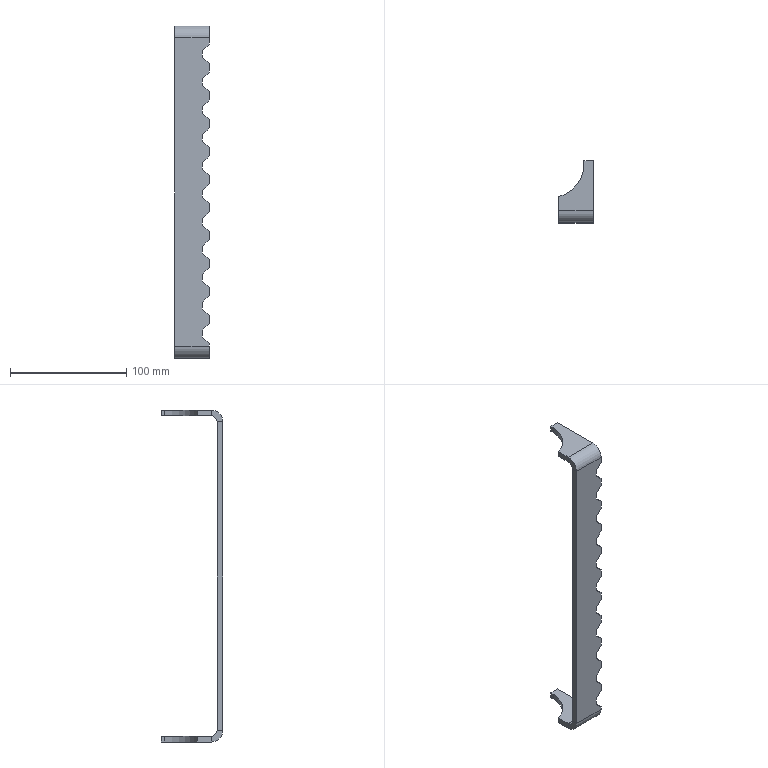Part | SolidWorks | features ICE 2, FlatPattern 1, SMBaseFlange 1, SheetMetal 1 | 1 solid | 70 faces | box 30 x 53 x 285 mm | volume 47239 mm3 | plane 64 | cylinder 6 | commonest cylinder face diameters 10 x2 20 x2 58 x2